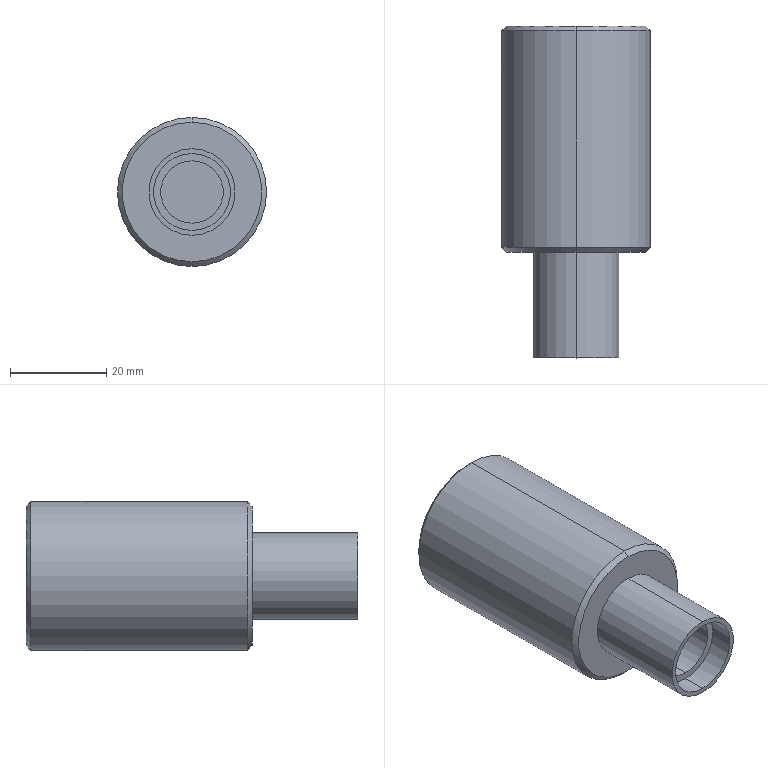Part | STEP file | PN_0009 Center JIG_Default | 1 solid | 17 faces | box 31 x 69 x 31 mm | volume 37981 mm3 | cylinder 8 | plane 5 | cone 4 | commonest cylinder face diameters 13 x2 16 x2 18 x2 31 x2
STEP:
#1=CARTESIAN_POINT('',(0.,0.,0.));
#2=DIRECTION('',(0.,0.,1.));
#3=DIRECTION('',(1.,0.,0.));
#4=AXIS2_PLACEMENT_3D('',#1,#2,#3);
#5=CARTESIAN_POINT('',(0.,22.,-14.5));
#6=VERTEX_POINT('',#5);
#7=CARTESIAN_POINT('',(0.,22.,14.5));
#8=VERTEX_POINT('',#7);
#9=CARTESIAN_POINT('',(0.,22.,0.));
#10=DIRECTION('',(0.,-1.,0.));
#11=DIRECTION('',(0.,0.,-1.));
#12=AXIS2_PLACEMENT_3D('',#9,#10,#11);
#13=CIRCLE('',#12,14.5);
#14=CARTESIAN_POINT('',(0.,22.,0.));
#15=DIRECTION('',(0.,1.,0.));
#16=DIRECTION('',(0.,0.,1.));
#17=AXIS2_PLACEMENT_3D('',#14,#15,#16);
#18=CONICAL_SURFACE('',#17,14.5,0.7854);
#19=CARTESIAN_POINT('',(3.142,0.));
#20=DIRECTION('',(-1.,0.));
#21=VECTOR('',#20,1.);
#22=LINE('',#19,#21);
#23=(GEOMETRIC_REPRESENTATION_CONTEXT(2)PARAMETRIC_REPRESENTATION_CONTEXT()REPRESENTATION_CONTEXT('',''));
#24=DEFINITIONAL_REPRESENTATION('',(#22),#23);
#25=PCURVE('',#18,#24);
#26=CARTESIAN_POINT('',(0.,22.,-15.5));
#27=DIRECTION('',(0.,-1.,0.));
#28=DIRECTION('',(0.,0.,-1.));
#29=AXIS2_PLACEMENT_3D('',#26,#27,#28);
#30=PLANE('',#29);
#31=CARTESIAN_POINT('',(-15.5,0.));
#32=DIRECTION('',(1.,0.));
#33=AXIS2_PLACEMENT_2D('',#31,#32);
#34=CIRCLE('',#33,14.5);
#35=(GEOMETRIC_REPRESENTATION_CONTEXT(2)PARAMETRIC_REPRESENTATION_CONTEXT()REPRESENTATION_CONTEXT('',''));
#36=DEFINITIONAL_REPRESENTATION('',(#34),#35);
#37=PCURVE('',#30,#36);
#38=SURFACE_CURVE('',#13,(#25,#37),.PCURVE_S1.);
#39=EDGE_CURVE('',#6,#8,#38,.T.);
#40=ORIENTED_EDGE('',*,*,#39,.F.);
#41=CARTESIAN_POINT('',(0.,23.,-15.5));
#42=VERTEX_POINT('',#41);
#43=CARTESIAN_POINT('',(0.,22.,-14.5));
#44=DIRECTION('',(0.,0.7071,-0.7071));
#45=VECTOR('',#44,1.);
#46=LINE('',#43,#45);
#47=CARTESIAN_POINT('',(3.142,0.));
#48=DIRECTION('',(0.,1.));
#49=VECTOR('',#48,1.);
#50=LINE('',#47,#49);
#51=(GEOMETRIC_REPRESENTATION_CONTEXT(2)PARAMETRIC_REPRESENTATION_CONTEXT()REPRESENTATION_CONTEXT('',''));
#52=DEFINITIONAL_REPRESENTATION('',(#50),#51);
#53=PCURVE('',#18,#52);
#54=CARTESIAN_POINT('',(0.,22.,0.));
#55=DIRECTION('',(0.,1.,0.));
#56=DIRECTION('',(0.,0.,1.));
#57=AXIS2_PLACEMENT_3D('',#54,#55,#56);
#58=CONICAL_SURFACE('',#57,14.5,0.7854);
#59=CARTESIAN_POINT('',(3.142,0.));
#60=DIRECTION('',(0.,1.));
#61=VECTOR('',#60,1.);
#62=LINE('',#59,#61);
#63=(GEOMETRIC_REPRESENTATION_CONTEXT(2)PARAMETRIC_REPRESENTATION_CONTEXT()REPRESENTATION_CONTEXT('',''));
#64=DEFINITIONAL_REPRESENTATION('',(#62),#63);
#65=PCURVE('',#58,#64);
#66=SURFACE_CURVE('',#46,(#53,#65),.PCURVE_S1.);
#67=EDGE_CURVE('',#6,#42,#66,.T.);
#68=ORIENTED_EDGE('',*,*,#67,.T.);
#69=CARTESIAN_POINT('',(0.,23.,15.5));
#70=VERTEX_POINT('',#69);
#71=CARTESIAN_POINT('',(0.,23.,0.));
#72=DIRECTION('',(0.,1.,0.));
#73=DIRECTION('',(0.,0.,-1.));
#74=AXIS2_PLACEMENT_3D('',#71,#72,#73);
#75=CIRCLE('',#74,15.5);
#76=CARTESIAN_POINT('',(-3.142,1.));
#77=DIRECTION('',(1.,0.));
#78=VECTOR('',#77,1.);
#79=LINE('',#76,#78);
#80=(GEOMETRIC_REPRESENTATION_CONTEXT(2)PARAMETRIC_REPRESENTATION_CONTEXT()REPRESENTATION_CONTEXT('',''));
#81=DEFINITIONAL_REPRESENTATION('',(#79),#80);
#82=PCURVE('',#18,#81);
#83=CARTESIAN_POINT('',(0.,-5.951,0.));
#84=DIRECTION('',(0.,-1.,0.));
#85=DIRECTION('',(0.,0.,-1.));
#86=AXIS2_PLACEMENT_3D('',#83,#84,#85);
#87=CYLINDRICAL_SURFACE('',#86,15.5);
#88=CARTESIAN_POINT('',(6.283,-28.951));
#89=DIRECTION('',(-1.,0.));
#90=VECTOR('',#89,1.);
#91=LINE('',#88,#90);
#92=(GEOMETRIC_REPRESENTATION_CONTEXT(2)PARAMETRIC_REPRESENTATION_CONTEXT()REPRESENTATION_CONTEXT('',''));
#93=DEFINITIONAL_REPRESENTATION('',(#91),#92);
#94=PCURVE('',#87,#93);
#95=SURFACE_CURVE('',#75,(#82,#94),.PCURVE_S1.);
#96=EDGE_CURVE('',#70,#42,#95,.T.);
#97=ORIENTED_EDGE('',*,*,#96,.F.);
#98=CARTESIAN_POINT('',(0.,22.,14.5));
#99=DIRECTION('',(0.,0.7071,0.7071));
#100=VECTOR('',#99,1.);
#101=LINE('',#98,#100);
#102=CARTESIAN_POINT('',(0.,0.));
#103=DIRECTION('',(0.,1.));
#104=VECTOR('',#103,1.);
#105=LINE('',#102,#104);
#106=(GEOMETRIC_REPRESENTATION_CONTEXT(2)PARAMETRIC_REPRESENTATION_CONTEXT()REPRESENTATION_CONTEXT('',''));
#107=DEFINITIONAL_REPRESENTATION('',(#105),#106);
#108=PCURVE('',#18,#107);
#109=CARTESIAN_POINT('',(6.283,0.));
#110=DIRECTION('',(0.,1.));
#111=VECTOR('',#110,1.);
#112=LINE('',#109,#111);
#113=(GEOMETRIC_REPRESENTATION_CONTEXT(2)PARAMETRIC_REPRESENTATION_CONTEXT()REPRESENTATION_CONTEXT('',''));
#114=DEFINITIONAL_REPRESENTATION('',(#112),#113);
#115=PCURVE('',#58,#114);
#116=SURFACE_CURVE('',#101,(#108,#115),.PCURVE_S1.);
#117=EDGE_CURVE('',#8,#70,#116,.T.);
#118=ORIENTED_EDGE('',*,*,#117,.F.);
#119=EDGE_LOOP('',(#40,#68,#97,#118));
#120=FACE_BOUND('',#119,.T.);
#121=ADVANCED_FACE('',(#120),#18,.T.);
#122=CARTESIAN_POINT('',(0.,69.,14.5));
#123=VERTEX_POINT('',#122);
#124=CARTESIAN_POINT('',(0.,69.,-14.5));
#125=VERTEX_POINT('',#124);
#126=CARTESIAN_POINT('',(0.,69.,0.));
#127=DIRECTION('',(0.,1.,0.));
#128=DIRECTION('',(0.,0.,1.));
#129=AXIS2_PLACEMENT_3D('',#126,#127,#128);
#130=CIRCLE('',#129,14.5);
#131=CARTESIAN_POINT('',(0.,68.,0.));
#132=DIRECTION('',(0.,-1.,0.));
#133=DIRECTION('',(0.,0.,-1.));
#134=AXIS2_PLACEMENT_3D('',#131,#132,#133);
#135=CONICAL_SURFACE('',#134,15.5,0.7854);
#136=CARTESIAN_POINT('',(3.142,-1.));
#137=DIRECTION('',(-1.,0.));
#138=VECTOR('',#137,1.);
#139=LINE('',#136,#138);
#140=(GEOMETRIC_REPRESENTATION_CONTEXT(2)PARAMETRIC_REPRESENTATION_CONTEXT()REPRESENTATION_CONTEXT('',''));
#141=DEFINITIONAL_REPRESENTATION('',(#139),#140);
#142=PCURVE('',#135,#141);
#143=CARTESIAN_POINT('',(0.,69.,-15.5));
#144=DIRECTION('',(0.,1.,0.));
#145=DIRECTION('',(0.,0.,1.));
#146=AXIS2_PLACEMENT_3D('',#143,#144,#145);
#147=PLANE('',#146);
#148=CARTESIAN_POINT('',(15.5,0.));
#149=DIRECTION('',(1.,0.));
#150=AXIS2_PLACEMENT_2D('',#148,#149);
#151=CIRCLE('',#150,14.5);
#152=(GEOMETRIC_REPRESENTATION_CONTEXT(2)PARAMETRIC_REPRESENTATION_CONTEXT()REPRESENTATION_CONTEXT('',''));
#153=DEFINITIONAL_REPRESENTATION('',(#151),#152);
#154=PCURVE('',#147,#153);
#155=SURFACE_CURVE('',#130,(#142,#154),.PCURVE_S1.);
#156=EDGE_CURVE('',#123,#125,#155,.T.);
#157=ORIENTED_EDGE('',*,*,#156,.F.);
#158=CARTESIAN_POINT('',(0.,68.,15.5));
#159=VERTEX_POINT('',#158);
#160=CARTESIAN_POINT('',(0.,68.,15.5));
#161=DIRECTION('',(0.,-0.7071,0.7071));
#162=VECTOR('',#161,1.);
#163=LINE('',#160,#162);
#164=CARTESIAN_POINT('',(3.142,0.));
#165=DIRECTION('',(0.,1.));
#166=VECTOR('',#165,1.);
#167=LINE('',#164,#166);
#168=(GEOMETRIC_REPRESENTATION_CONTEXT(2)PARAMETRIC_REPRESENTATION_CONTEXT()REPRESENTATION_CONTEXT('',''));
#169=DEFINITIONAL_REPRESENTATION('',(#167),#168);
#170=PCURVE('',#135,#169);
#171=CARTESIAN_POINT('',(0.,68.,0.));
#172=DIRECTION('',(0.,-1.,0.));
#173=DIRECTION('',(0.,0.,-1.));
#174=AXIS2_PLACEMENT_3D('',#171,#172,#173);
#175=CONICAL_SURFACE('',#174,15.5,0.7854);
#176=CARTESIAN_POINT('',(3.142,0.));
#177=DIRECTION('',(0.,1.));
#178=VECTOR('',#177,1.);
#179=LINE('',#176,#178);
#180=(GEOMETRIC_REPRESENTATION_CONTEXT(2)PARAMETRIC_REPRESENTATION_CONTEXT()REPRESENTATION_CONTEXT('',''));
#181=DEFINITIONAL_REPRESENTATION('',(#179),#180);
#182=PCURVE('',#175,#181);
#183=SURFACE_CURVE('',#163,(#170,#182),.PCURVE_S1.);
#184=EDGE_CURVE('',#123,#159,#183,.T.);
#185=ORIENTED_EDGE('',*,*,#184,.T.);
#186=CARTESIAN_POINT('',(0.,68.,-15.5));
#187=VERTEX_POINT('',#186);
#188=CARTESIAN_POINT('',(0.,68.,0.));
#189=DIRECTION('',(0.,-1.,0.));
#190=DIRECTION('',(0.,0.,1.));
#191=AXIS2_PLACEMENT_3D('',#188,#189,#190);
#192=CIRCLE('',#191,15.5);
#193=CARTESIAN_POINT('',(-3.142,0.));
#194=DIRECTION('',(1.,0.));
#195=VECTOR('',#194,1.);
#196=LINE('',#193,#195);
#197=(GEOMETRIC_REPRESENTATION_CONTEXT(2)PARAMETRIC_REPRESENTATION_CONTEXT()REPRESENTATION_CONTEXT('',''));
#198=DEFINITIONAL_REPRESENTATION('',(#196),#197);
#199=PCURVE('',#135,#198);
#200=CARTESIAN_POINT('',(-3.142,-73.951));
#201=DIRECTION('',(1.,0.));
#202=VECTOR('',#201,1.);
#203=LINE('',#200,#202);
#204=(GEOMETRIC_REPRESENTATION_CONTEXT(2)PARAMETRIC_REPRESENTATION_CONTEXT()REPRESENTATION_CONTEXT('',''));
#205=DEFINITIONAL_REPRESENTATION('',(#203),#204);
#206=PCURVE('',#87,#205);
#207=SURFACE_CURVE('',#192,(#199,#206),.PCURVE_S1.);
#208=EDGE_CURVE('',#187,#159,#207,.T.);
#209=ORIENTED_EDGE('',*,*,#208,.F.);
#210=CARTESIAN_POINT('',(0.,68.,-15.5));
#211=DIRECTION('',(0.,-0.7071,-0.7071));
#212=VECTOR('',#211,1.);
#213=LINE('',#210,#212);
#214=CARTESIAN_POINT('',(0.,0.));
#215=DIRECTION('',(0.,1.));
#216=VECTOR('',#215,1.);
#217=LINE('',#214,#216);
#218=(GEOMETRIC_REPRESENTATION_CONTEXT(2)PARAMETRIC_REPRESENTATION_CONTEXT()REPRESENTATION_CONTEXT('',''));
#219=DEFINITIONAL_REPRESENTATION('',(#217),#218);
#220=PCURVE('',#135,#219);
#221=CARTESIAN_POINT('',(6.283,0.));
#222=DIRECTION('',(0.,1.));
#223=VECTOR('',#222,1.);
#224=LINE('',#221,#223);
#225=(GEOMETRIC_REPRESENTATION_CONTEXT(2)PARAMETRIC_REPRESENTATION_CONTEXT()REPRESENTATION_CONTEXT('',''));
#226=DEFINITIONAL_REPRESENTATION('',(#224),#225);
#227=PCURVE('',#175,#226);
#228=SURFACE_CURVE('',#213,(#220,#227),.PCURVE_S1.);
#229=EDGE_CURVE('',#125,#187,#228,.T.);
#230=ORIENTED_EDGE('',*,*,#229,.F.);
#231=EDGE_LOOP('',(#157,#185,#209,#230));
#232=FACE_BOUND('',#231,.T.);
#233=ADVANCED_FACE('',(#232),#135,.T.);
#234=CARTESIAN_POINT('',(0.,20.,-6.5));
#235=VERTEX_POINT('',#234);
#236=CARTESIAN_POINT('',(0.,5.,-6.5));
#237=VERTEX_POINT('',#236);
#238=CARTESIAN_POINT('',(0.,20.,-6.5));
#239=DIRECTION('',(0.,-1.,0.));
#240=VECTOR('',#239,1.);
#241=LINE('',#238,#240);
#242=CARTESIAN_POINT('',(0.,20.,0.));
#243=DIRECTION('',(0.,-1.,0.));
#244=DIRECTION('',(0.,0.,-1.));
#245=AXIS2_PLACEMENT_3D('',#242,#243,#244);
#246=CYLINDRICAL_SURFACE('',#245,6.5);
#247=CARTESIAN_POINT('',(6.283,0.));
#248=DIRECTION('',(0.,1.));
#249=VECTOR('',#248,1.);
#250=LINE('',#247,#249);
#251=(GEOMETRIC_REPRESENTATION_CONTEXT(2)PARAMETRIC_REPRESENTATION_CONTEXT()REPRESENTATION_CONTEXT('',''));
#252=DEFINITIONAL_REPRESENTATION('',(#250),#251);
#253=PCURVE('',#246,#252);
#254=CARTESIAN_POINT('',(0.,20.,0.));
#255=DIRECTION('',(0.,-1.,0.));
#256=DIRECTION('',(0.,0.,-1.));
#257=AXIS2_PLACEMENT_3D('',#254,#255,#256);
#258=CYLINDRICAL_SURFACE('',#257,6.5);
#259=CARTESIAN_POINT('',(0.,0.));
#260=DIRECTION('',(0.,1.));
#261=VECTOR('',#260,1.);
#262=LINE('',#259,#261);
#263=(GEOMETRIC_REPRESENTATION_CONTEXT(2)PARAMETRIC_REPRESENTATION_CONTEXT()REPRESENTATION_CONTEXT('',''));
#264=DEFINITIONAL_REPRESENTATION('',(#262),#263);
#265=PCURVE('',#258,#264);
#266=SURFACE_CURVE('',#241,(#253,#265),.PCURVE_S1.);
#267=EDGE_CURVE('',#235,#237,#266,.T.);
#268=ORIENTED_EDGE('',*,*,#267,.T.);
#269=CARTESIAN_POINT('',(0.,5.,6.5));
#270=VERTEX_POINT('',#269);
#271=CARTESIAN_POINT('',(0.,5.,0.));
#272=DIRECTION('',(0.,-1.,0.));
#273=DIRECTION('',(0.,0.,-1.));
#274=AXIS2_PLACEMENT_3D('',#271,#272,#273);
#275=CIRCLE('',#274,6.5);
#276=CARTESIAN_POINT('',(0.,15.));
#277=DIRECTION('',(1.,0.));
#278=VECTOR('',#277,1.);
#279=LINE('',#276,#278);
#280=(GEOMETRIC_REPRESENTATION_CONTEXT(2)PARAMETRIC_REPRESENTATION_CONTEXT()REPRESENTATION_CONTEXT('',''));
#281=DEFINITIONAL_REPRESENTATION('',(#279),#280);
#282=PCURVE('',#246,#281);
#283=CARTESIAN_POINT('',(0.,5.,0.));
#284=DIRECTION('',(0.,-1.,0.));
#285=DIRECTION('',(0.,0.,-1.));
#286=AXIS2_PLACEMENT_3D('',#283,#284,#285);
#287=PLANE('',#286);
#288=CARTESIAN_POINT('',(0.,0.));
#289=DIRECTION('',(1.,0.));
#290=AXIS2_PLACEMENT_2D('',#288,#289);
#291=CIRCLE('',#290,6.5);
#292=(GEOMETRIC_REPRESENTATION_CONTEXT(2)PARAMETRIC_REPRESENTATION_CONTEXT()REPRESENTATION_CONTEXT('',''));
#293=DEFINITIONAL_REPRESENTATION('',(#291),#292);
#294=PCURVE('',#287,#293);
#295=SURFACE_CURVE('',#275,(#282,#294),.PCURVE_S1.);
#296=EDGE_CURVE('',#270,#237,#295,.T.);
#297=ORIENTED_EDGE('',*,*,#296,.F.);
#298=CARTESIAN_POINT('',(0.,20.,6.5));
#299=VERTEX_POINT('',#298);
#300=CARTESIAN_POINT('',(0.,20.,6.5));
#301=DIRECTION('',(0.,-1.,0.));
#302=VECTOR('',#301,1.);
#303=LINE('',#300,#302);
#304=CARTESIAN_POINT('',(3.142,0.));
#305=DIRECTION('',(0.,1.));
#306=VECTOR('',#305,1.);
#307=LINE('',#304,#306);
#308=(GEOMETRIC_REPRESENTATION_CONTEXT(2)PARAMETRIC_REPRESENTATION_CONTEXT()REPRESENTATION_CONTEXT('',''));
#309=DEFINITIONAL_REPRESENTATION('',(#307),#308);
#310=PCURVE('',#246,#309);
#311=CARTESIAN_POINT('',(3.142,0.));
#312=DIRECTION('',(0.,1.));
#313=VECTOR('',#312,1.);
#314=LINE('',#311,#313);
#315=(GEOMETRIC_REPRESENTATION_CONTEXT(2)PARAMETRIC_REPRESENTATION_CONTEXT()REPRESENTATION_CONTEXT('',''));
#316=DEFINITIONAL_REPRESENTATION('',(#314),#315);
#317=PCURVE('',#258,#316);
#318=SURFACE_CURVE('',#303,(#310,#317),.PCURVE_S1.);
#319=EDGE_CURVE('',#299,#270,#318,.T.);
#320=ORIENTED_EDGE('',*,*,#319,.F.);
#321=CARTESIAN_POINT('',(0.,20.,0.));
#322=DIRECTION('',(0.,-1.,0.));
#323=DIRECTION('',(0.,0.,-1.));
#324=AXIS2_PLACEMENT_3D('',#321,#322,#323);
#325=CIRCLE('',#324,6.5);
#326=CARTESIAN_POINT('',(0.,0.));
#327=DIRECTION('',(1.,0.));
#328=VECTOR('',#327,1.);
#329=LINE('',#326,#328);
#330=(GEOMETRIC_REPRESENTATION_CONTEXT(2)PARAMETRIC_REPRESENTATION_CONTEXT()REPRESENTATION_CONTEXT('',''));
#331=DEFINITIONAL_REPRESENTATION('',(#329),#330);
#332=PCURVE('',#246,#331);
#333=CARTESIAN_POINT('',(0.,20.,0.));
#334=DIRECTION('',(0.,-1.,0.));
#335=DIRECTION('',(0.,0.,-1.));
#336=AXIS2_PLACEMENT_3D('',#333,#334,#335);
#337=PLANE('',#336);
#338=CARTESIAN_POINT('',(0.,0.));
#339=DIRECTION('',(1.,0.));
#340=AXIS2_PLACEMENT_2D('',#338,#339);
#341=CIRCLE('',#340,6.5);
#342=(GEOMETRIC_REPRESENTATION_CONTEXT(2)PARAMETRIC_REPRESENTATION_CONTEXT()REPRESENTATION_CONTEXT('',''));
#343=DEFINITIONAL_REPRESENTATION('',(#341),#342);
#344=PCURVE('',#337,#343);
#345=SURFACE_CURVE('',#325,(#332,#344),.PCURVE_S1.);
#346=EDGE_CURVE('',#299,#235,#345,.T.);
#347=ORIENTED_EDGE('',*,*,#346,.T.);
#348=EDGE_LOOP('',(#268,#297,#320,#347));
#349=FACE_BOUND('',#348,.F.);
#350=ADVANCED_FACE('',(#349),#246,.F.);
#351=CARTESIAN_POINT('',(0.,5.,-8.));
#352=VERTEX_POINT('',#351);
#353=CARTESIAN_POINT('',(0.,0.,-8.));
#354=VERTEX_POINT('',#353);
#355=CARTESIAN_POINT('',(0.,5.,-8.));
#356=DIRECTION('',(0.,-1.,0.));
#357=VECTOR('',#356,1.);
#358=LINE('',#355,#357);
#359=CARTESIAN_POINT('',(0.,5.,0.));
#360=DIRECTION('',(0.,-1.,0.));
#361=DIRECTION('',(0.,0.,-1.));
#362=AXIS2_PLACEMENT_3D('',#359,#360,#361);
#363=CYLINDRICAL_SURFACE('',#362,8.);
#364=CARTESIAN_POINT('',(6.283,0.));
#365=DIRECTION('',(0.,1.));
#366=VECTOR('',#365,1.);
#367=LINE('',#364,#366);
#368=(GEOMETRIC_REPRESENTATION_CONTEXT(2)PARAMETRIC_REPRESENTATION_CONTEXT()REPRESENTATION_CONTEXT('',''));
#369=DEFINITIONAL_REPRESENTATION('',(#367),#368);
#370=PCURVE('',#363,#369);
#371=CARTESIAN_POINT('',(0.,5.,0.));
#372=DIRECTION('',(0.,-1.,0.));
#373=DIRECTION('',(0.,0.,-1.));
#374=AXIS2_PLACEMENT_3D('',#371,#372,#373);
#375=CYLINDRICAL_SURFACE('',#374,8.);
#376=CARTESIAN_POINT('',(0.,0.));
#377=DIRECTION('',(0.,1.));
#378=VECTOR('',#377,1.);
#379=LINE('',#376,#378);
#380=(GEOMETRIC_REPRESENTATION_CONTEXT(2)PARAMETRIC_REPRESENTATION_CONTEXT()REPRESENTATION_CONTEXT('',''));
#381=DEFINITIONAL_REPRESENTATION('',(#379),#380);
#382=PCURVE('',#375,#381);
#383=SURFACE_CURVE('',#358,(#370,#382),.PCURVE_S1.);
#384=EDGE_CURVE('',#352,#354,#383,.T.);
#385=ORIENTED_EDGE('',*,*,#384,.T.);
#386=CARTESIAN_POINT('',(0.,0.,8.));
#387=VERTEX_POINT('',#386);
#388=CARTESIAN_POINT('',(0.,0.,0.));
#389=DIRECTION('',(0.,-1.,0.));
#390=DIRECTION('',(0.,0.,-1.));
#391=AXIS2_PLACEMENT_3D('',#388,#389,#390);
#392=CIRCLE('',#391,8.);
#393=CARTESIAN_POINT('',(0.,5.));
#394=DIRECTION('',(1.,0.));
#395=VECTOR('',#394,1.);
#396=LINE('',#393,#395);
#397=(GEOMETRIC_REPRESENTATION_CONTEXT(2)PARAMETRIC_REPRESENTATION_CONTEXT()REPRESENTATION_CONTEXT('',''));
#398=DEFINITIONAL_REPRESENTATION('',(#396),#397);
#399=PCURVE('',#363,#398);
#400=CARTESIAN_POINT('',(0.,0.,-9.));
#401=DIRECTION('',(0.,-1.,0.));
#402=DIRECTION('',(0.,0.,-1.));
#403=AXIS2_PLACEMENT_3D('',#400,#401,#402);
#404=PLANE('',#403);
#405=CARTESIAN_POINT('',(-9.,0.));
#406=DIRECTION('',(1.,0.));
#407=AXIS2_PLACEMENT_2D('',#405,#406);
#408=CIRCLE('',#407,8.);
#409=(GEOMETRIC_REPRESENTATION_CONTEXT(2)PARAMETRIC_REPRESENTATION_CONTEXT()REPRESENTATION_CONTEXT('',''));
#410=DEFINITIONAL_REPRESENTATION('',(#408),#409);
#411=PCURVE('',#404,#410);
#412=SURFACE_CURVE('',#392,(#399,#411),.PCURVE_S1.);
#413=EDGE_CURVE('',#387,#354,#412,.T.);
#414=ORIENTED_EDGE('',*,*,#413,.F.);
#415=CARTESIAN_POINT('',(0.,5.,8.));
#416=VERTEX_POINT('',#415);
#417=CARTESIAN_POINT('',(0.,5.,8.));
#418=DIRECTION('',(0.,-1.,0.));
#419=VECTOR('',#418,1.);
#420=LINE('',#417,#419);
#421=CARTESIAN_POINT('',(3.142,0.));
#422=DIRECTION('',(0.,1.));
#423=VECTOR('',#422,1.);
#424=LINE('',#421,#423);
#425=(GEOMETRIC_REPRESENTATION_CONTEXT(2)PARAMETRIC_REPRESENTATION_CONTEXT()REPRESENTATION_CONTEXT('',''));
#426=DEFINITIONAL_REPRESENTATION('',(#424),#425);
#427=PCURVE('',#363,#426);
#428=CARTESIAN_POINT('',(3.142,0.));
#429=DIRECTION('',(0.,1.));
#430=VECTOR('',#429,1.);
#431=LINE('',#428,#430);
#432=(GEOMETRIC_REPRESENTATION_CONTEXT(2)PARAMETRIC_REPRESENTATION_CONTEXT()REPRESENTATION_CONTEXT('',''));
#433=DEFINITIONAL_REPRESENTATION('',(#431),#432);
#434=PCURVE('',#375,#433);
#435=SURFACE_CURVE('',#420,(#427,#434),.PCURVE_S1.);
#436=EDGE_CURVE('',#416,#387,#435,.T.);
#437=ORIENTED_EDGE('',*,*,#436,.F.);
#438=CARTESIAN_POINT('',(0.,5.,0.));
#439=DIRECTION('',(0.,-1.,0.));
#440=DIRECTION('',(0.,0.,-1.));
#441=AXIS2_PLACEMENT_3D('',#438,#439,#440);
#442=CIRCLE('',#441,8.);
#443=CARTESIAN_POINT('',(0.,0.));
#444=DIRECTION('',(1.,0.));
#445=VECTOR('',#444,1.);
#446=LINE('',#443,#445);
#447=(GEOMETRIC_REPRESENTATION_CONTEXT(2)PARAMETRIC_REPRESENTATION_CONTEXT()REPRESENTATION_CONTEXT('',''));
#448=DEFINITIONAL_REPRESENTATION('',(#446),#447);
#449=PCURVE('',#363,#448);
#450=CARTESIAN_POINT('',(0.,0.));
#451=DIRECTION('',(1.,0.));
#452=AXIS2_PLACEMENT_2D('',#450,#451);
#453=CIRCLE('',#452,8.);
#454=(GEOMETRIC_REPRESENTATION_CONTEXT(2)PARAMETRIC_REPRESENTATION_CONTEXT()REPRESENTATION_CONTEXT('',''));
#455=DEFINITIONAL_REPRESENTATION('',(#453),#454);
#456=PCURVE('',#287,#455);
#457=SURFACE_CURVE('',#442,(#449,#456),.PCURVE_S1.);
#458=EDGE_CURVE('',#416,#352,#457,.T.);
#459=ORIENTED_EDGE('',*,*,#458,.T.);
#460=EDGE_LOOP('',(#385,#414,#437,#459));
#461=FACE_BOUND('',#460,.F.);
#462=ADVANCED_FACE('',(#461),#363,.F.);
#463=ORIENTED_EDGE('',*,*,#208,.T.);
#464=CARTESIAN_POINT('',(0.,-5.951,15.5));
#465=DIRECTION('',(0.,-1.,0.));
#466=VECTOR('',#465,1.);
#467=LINE('',#464,#466);
#468=CARTESIAN_POINT('',(3.142,0.));
#469=DIRECTION('',(0.,1.));
#470=VECTOR('',#469,1.);
#471=LINE('',#468,#470);
#472=(GEOMETRIC_REPRESENTATION_CONTEXT(2)PARAMETRIC_REPRESENTATION_CONTEXT()REPRESENTATION_CONTEXT('',''));
#473=DEFINITIONAL_REPRESENTATION('',(#471),#472);
#474=PCURVE('',#87,#473);
#475=CARTESIAN_POINT('',(0.,-5.951,0.));
#476=DIRECTION('',(0.,-1.,0.));
#477=DIRECTION('',(0.,0.,-1.));
#478=AXIS2_PLACEMENT_3D('',#475,#476,#477);
#479=CYLINDRICAL_SURFACE('',#478,15.5);
#480=CARTESIAN_POINT('',(3.142,0.));
#481=DIRECTION('',(0.,1.));
#482=VECTOR('',#481,1.);
#483=LINE('',#480,#482);
#484=(GEOMETRIC_REPRESENTATION_CONTEXT(2)PARAMETRIC_REPRESENTATION_CONTEXT()REPRESENTATION_CONTEXT('',''));
#485=DEFINITIONAL_REPRESENTATION('',(#483),#484);
#486=PCURVE('',#479,#485);
#487=SURFACE_CURVE('',#467,(#474,#486),.PCURVE_S1.);
#488=EDGE_CURVE('',#159,#70,#487,.T.);
#489=ORIENTED_EDGE('',*,*,#488,.T.);
#490=ORIENTED_EDGE('',*,*,#96,.T.);
#491=CARTESIAN_POINT('',(0.,-5.951,-15.5));
#492=DIRECTION('',(0.,-1.,0.));
#493=VECTOR('',#492,1.);
#494=LINE('',#491,#493);
#495=CARTESIAN_POINT('',(0.,0.));
#496=DIRECTION('',(0.,1.));
#497=VECTOR('',#496,1.);
#498=LINE('',#495,#497);
#499=(GEOMETRIC_REPRESENTATION_CONTEXT(2)PARAMETRIC_REPRESENTATION_CONTEXT()REPRESENTATION_CONTEXT('',''));
#500=DEFINITIONAL_REPRESENTATION('',(#498),#499);
#501=PCURVE('',#87,#500);
#502=CARTESIAN_POINT('',(6.283,0.));
#503=DIRECTION('',(0.,1.));
#504=VECTOR('',#503,1.);
#505=LINE('',#502,#504);
#506=(GEOMETRIC_REPRESENTATION_CONTEXT(2)PARAMETRIC_REPRESENTATION_CONTEXT()REPRESENTATION_CONTEXT('',''));
#507=DEFINITIONAL_REPRESENTATION('',(#505),#506);
#508=PCURVE('',#479,#507);
#509=SURFACE_CURVE('',#494,(#501,#508),.PCURVE_S1.);
#510=EDGE_CURVE('',#187,#42,#509,.T.);
#511=ORIENTED_EDGE('',*,*,#510,.F.);
#512=EDGE_LOOP('',(#463,#489,#490,#511));
#513=FACE_BOUND('',#512,.T.);
#514=ADVANCED_FACE('',(#513),#87,.T.);
#515=CARTESIAN_POINT('',(0.,22.,-9.));
#516=VERTEX_POINT('',#515);
#517=CARTESIAN_POINT('',(0.,22.,9.));
#518=VERTEX_POINT('',#517);
#519=CARTESIAN_POINT('',(0.,22.,0.));
#520=DIRECTION('',(0.,-1.,0.));
#521=DIRECTION('',(0.,0.,-1.));
#522=AXIS2_PLACEMENT_3D('',#519,#520,#521);
#523=CIRCLE('',#522,9.);
#524=CARTESIAN_POINT('',(0.,-5.951,0.));
#525=DIRECTION('',(0.,-1.,0.));
#526=DIRECTION('',(0.,0.,-1.));
#527=AXIS2_PLACEMENT_3D('',#524,#525,#526);
#528=CYLINDRICAL_SURFACE('',#527,9.);
#529=CARTESIAN_POINT('',(0.,-27.951));
#530=DIRECTION('',(1.,0.));
#531=VECTOR('',#530,1.);
#532=LINE('',#529,#531);
#533=(GEOMETRIC_REPRESENTATION_CONTEXT(2)PARAMETRIC_REPRESENTATION_CONTEXT()REPRESENTATION_CONTEXT('',''));
#534=DEFINITIONAL_REPRESENTATION('',(#532),#533);
#535=PCURVE('',#528,#534);
#536=CARTESIAN_POINT('',(-15.5,0.));
#537=DIRECTION('',(1.,0.));
#538=AXIS2_PLACEMENT_2D('',#536,#537);
#539=CIRCLE('',#538,9.);
#540=(GEOMETRIC_REPRESENTATION_CONTEXT(2)PARAMETRIC_REPRESENTATION_CONTEXT()REPRESENTATION_CONTEXT('',''));
#541=DEFINITIONAL_REPRESENTATION('',(#539),#540);
#542=PCURVE('',#30,#541);
#543=SURFACE_CURVE('',#523,(#535,#542),.PCURVE_S1.);
#544=EDGE_CURVE('',#516,#518,#543,.T.);
#545=ORIENTED_EDGE('',*,*,#544,.T.);
#546=CARTESIAN_POINT('',(0.,0.,9.));
#547=VERTEX_POINT('',#546);
#548=CARTESIAN_POINT('',(0.,-5.951,9.));
#549=DIRECTION('',(0.,-1.,0.));
#550=VECTOR('',#549,1.);
#551=LINE('',#548,#550);
#552=CARTESIAN_POINT('',(3.142,0.));
#553=DIRECTION('',(0.,1.));
#554=VECTOR('',#553,1.);
#555=LINE('',#552,#554);
#556=(GEOMETRIC_REPRESENTATION_CONTEXT(2)PARAMETRIC_REPRESENTATION_CONTEXT()REPRESENTATION_CONTEXT('',''));
#557=DEFINITIONAL_REPRESENTATION('',(#555),#556);
#558=PCURVE('',#528,#557);
#559=CARTESIAN_POINT('',(0.,-5.951,0.));
#560=DIRECTION('',(0.,-1.,0.));
#561=DIRECTION('',(0.,0.,-1.));
#562=AXIS2_PLACEMENT_3D('',#559,#560,#561);
#563=CYLINDRICAL_SURFACE('',#562,9.);
#564=CARTESIAN_POINT('',(3.142,0.));
#565=DIRECTION('',(0.,1.));
#566=VECTOR('',#565,1.);
#567=LINE('',#564,#566);
#568=(GEOMETRIC_REPRESENTATION_CONTEXT(2)PARAMETRIC_REPRESENTATION_CONTEXT()REPRESENTATION_CONTEXT('',''));
#569=DEFINITIONAL_REPRESENTATION('',(#567),#568);
#570=PCURVE('',#563,#569);
#571=SURFACE_CURVE('',#551,(#558,#570),.PCURVE_S1.);
#572=EDGE_CURVE('',#518,#547,#571,.T.);
#573=ORIENTED_EDGE('',*,*,#572,.T.);
#574=CARTESIAN_POINT('',(0.,0.,-9.));
#575=VERTEX_POINT('',#574);
#576=CARTESIAN_POINT('',(0.,0.,0.));
#577=DIRECTION('',(0.,-1.,0.));
#578=DIRECTION('',(0.,0.,-1.));
#579=AXIS2_PLACEMENT_3D('',#576,#577,#578);
#580=CIRCLE('',#579,9.);
#581=CARTESIAN_POINT('',(0.,-5.951));
#582=DIRECTION('',(1.,0.));
#583=VECTOR('',#582,1.);
#584=LINE('',#581,#583);
#585=(GEOMETRIC_REPRESENTATION_CONTEXT(2)PARAMETRIC_REPRESENTATION_CONTEXT()REPRESENTATION_CONTEXT('',''));
#586=DEFINITIONAL_REPRESENTATION('',(#584),#585);
#587=PCURVE('',#528,#586);
#588=CARTESIAN_POINT('',(-9.,0.));
#589=DIRECTION('',(1.,0.));
#590=AXIS2_PLACEMENT_2D('',#588,#589);
#591=CIRCLE('',#590,9.);
#592=(GEOMETRIC_REPRESENTATION_CONTEXT(2)PARAMETRIC_REPRESENTATION_CONTEXT()REPRESENTATION_CONTEXT('',''));
#593=DEFINITIONAL_REPRESENTATION('',(#591),#592);
#594=PCURVE('',#404,#593);
#595=SURFACE_CURVE('',#580,(#587,#594),.PCURVE_S1.);
#596=EDGE_CURVE('',#575,#547,#595,.T.);
#597=ORIENTED_EDGE('',*,*,#596,.F.);
#598=CARTESIAN_POINT('',(0.,-5.951,-9.));
#599=DIRECTION('',(0.,-1.,0.));
#600=VECTOR('',#599,1.);
#601=LINE('',#598,#600);
#602=CARTESIAN_POINT('',(0.,0.));
#603=DIRECTION('',(0.,1.));
#604=VECTOR('',#603,1.);
#605=LINE('',#602,#604);
#606=(GEOMETRIC_REPRESENTATION_CONTEXT(2)PARAMETRIC_REPRESENTATION_CONTEXT()REPRESENTATION_CONTEXT('',''));
#607=DEFINITIONAL_REPRESENTATION('',(#605),#606);
#608=PCURVE('',#528,#607);
#609=CARTESIAN_POINT('',(6.283,0.));
#610=DIRECTION('',(0.,1.));
#611=VECTOR('',#610,1.);
#612=LINE('',#609,#611);
#613=(GEOMETRIC_REPRESENTATION_CONTEXT(2)PARAMETRIC_REPRESENTATION_CONTEXT()REPRESENTATION_CONTEXT('',''));
#614=DEFINITIONAL_REPRESENTATION('',(#612),#613);
#615=PCURVE('',#563,#614);
#616=SURFACE_CURVE('',#601,(#608,#615),.PCURVE_S1.);
#617=EDGE_CURVE('',#516,#575,#616,.T.);
#618=ORIENTED_EDGE('',*,*,#617,.F.);
#619=EDGE_LOOP('',(#545,#573,#597,#618));
#620=FACE_BOUND('',#619,.T.);
#621=ADVANCED_FACE('',(#620),#528,.T.);
#622=CARTESIAN_POINT('',(0.,0.,0.));
#623=DIRECTION('',(0.,-1.,0.));
#624=DIRECTION('',(0.,0.,-1.));
#625=AXIS2_PLACEMENT_3D('',#622,#623,#624);
#626=CIRCLE('',#625,8.);
#627=CARTESIAN_POINT('',(-9.,0.));
#628=DIRECTION('',(1.,0.));
#629=AXIS2_PLACEMENT_2D('',#627,#628);
#630=CIRCLE('',#629,8.);
#631=(GEOMETRIC_REPRESENTATION_CONTEXT(2)PARAMETRIC_REPRESENTATION_CONTEXT()REPRESENTATION_CONTEXT('',''));
#632=DEFINITIONAL_REPRESENTATION('',(#630),#631);
#633=PCURVE('',#404,#632);
#634=CARTESIAN_POINT('',(0.,5.));
#635=DIRECTION('',(1.,0.));
#636=VECTOR('',#635,1.);
#637=LINE('',#634,#636);
#638=(GEOMETRIC_REPRESENTATION_CONTEXT(2)PARAMETRIC_REPRESENTATION_CONTEXT()REPRESENTATION_CONTEXT('',''));
#639=DEFINITIONAL_REPRESENTATION('',(#637),#638);
#640=PCURVE('',#375,#639);
#641=SURFACE_CURVE('',#626,(#633,#640),.PCURVE_S1.);
#642=EDGE_CURVE('',#354,#387,#641,.T.);
#643=ORIENTED_EDGE('',*,*,#642,.F.);
#644=ORIENTED_EDGE('',*,*,#413,.F.);
#645=EDGE_LOOP('',(#643,#644));
#646=FACE_BOUND('',#645,.T.);
#647=ORIENTED_EDGE('',*,*,#596,.T.);
#648=CARTESIAN_POINT('',(0.,0.,0.));
#649=DIRECTION('',(0.,-1.,0.));
#650=DIRECTION('',(0.,0.,-1.));
#651=AXIS2_PLACEMENT_3D('',#648,#649,#650);
#652=CIRCLE('',#651,9.);
#653=CARTESIAN_POINT('',(-9.,0.));
#654=DIRECTION('',(1.,0.));
#655=AXIS2_PLACEMENT_2D('',#653,#654);
#656=CIRCLE('',#655,9.);
#657=(GEOMETRIC_REPRESENTATION_CONTEXT(2)PARAMETRIC_REPRESENTATION_CONTEXT()REPRESENTATION_CONTEXT('',''));
#658=DEFINITIONAL_REPRESENTATION('',(#656),#657);
#659=PCURVE('',#404,#658);
#660=CARTESIAN_POINT('',(0.,-5.951));
#661=DIRECTION('',(1.,0.));
#662=VECTOR('',#661,1.);
#663=LINE('',#660,#662);
#664=(GEOMETRIC_REPRESENTATION_CONTEXT(2)PARAMETRIC_REPRESENTATION_CONTEXT()REPRESENTATION_CONTEXT('',''));
#665=DEFINITIONAL_REPRESENTATION('',(#663),#664);
#666=PCURVE('',#563,#665);
#667=SURFACE_CURVE('',#652,(#659,#666),.PCURVE_S1.);
#668=EDGE_CURVE('',#547,#575,#667,.T.);
#669=ORIENTED_EDGE('',*,*,#668,.T.);
#670=EDGE_LOOP('',(#647,#669));
#671=FACE_BOUND('',#670,.T.);
#672=ADVANCED_FACE('',(#646,#671),#404,.T.);
#673=ORIENTED_EDGE('',*,*,#572,.F.);
#674=CARTESIAN_POINT('',(0.,22.,0.));
#675=DIRECTION('',(0.,-1.,0.));
#676=DIRECTION('',(0.,0.,-1.));
#677=AXIS2_PLACEMENT_3D('',#674,#675,#676);
#678=CIRCLE('',#677,9.);
#679=CARTESIAN_POINT('',(0.,-27.951));
#680=DIRECTION('',(1.,0.));
#681=VECTOR('',#680,1.);
#682=LINE('',#679,#681);
#683=(GEOMETRIC_REPRESENTATION_CONTEXT(2)PARAMETRIC_REPRESENTATION_CONTEXT()REPRESENTATION_CONTEXT('',''));
#684=DEFINITIONAL_REPRESENTATION('',(#682),#683);
#685=PCURVE('',#563,#684);
#686=CARTESIAN_POINT('',(-15.5,0.));
#687=DIRECTION('',(1.,0.));
#688=AXIS2_PLACEMENT_2D('',#686,#687);
#689=CIRCLE('',#688,9.);
#690=(GEOMETRIC_REPRESENTATION_CONTEXT(2)PARAMETRIC_REPRESENTATION_CONTEXT()REPRESENTATION_CONTEXT('',''));
#691=DEFINITIONAL_REPRESENTATION('',(#689),#690);
#692=PCURVE('',#30,#691);
#693=SURFACE_CURVE('',#678,(#685,#692),.PCURVE_S1.);
#694=EDGE_CURVE('',#518,#516,#693,.T.);
#695=ORIENTED_EDGE('',*,*,#694,.T.);
#696=ORIENTED_EDGE('',*,*,#617,.T.);
#697=ORIENTED_EDGE('',*,*,#668,.F.);
#698=EDGE_LOOP('',(#673,#695,#696,#697));
#699=FACE_BOUND('',#698,.T.);
#700=ADVANCED_FACE('',(#699),#563,.T.);
#701=CARTESIAN_POINT('',(0.,22.,0.));
#702=DIRECTION('',(0.,-1.,0.));
#703=DIRECTION('',(0.,0.,-1.));
#704=AXIS2_PLACEMENT_3D('',#701,#702,#703);
#705=CIRCLE('',#704,14.5);
#706=CARTESIAN_POINT('',(-15.5,0.));
#707=DIRECTION('',(1.,0.));
#708=AXIS2_PLACEMENT_2D('',#706,#707);
#709=CIRCLE('',#708,14.5);
#710=(GEOMETRIC_REPRESENTATION_CONTEXT(2)PARAMETRIC_REPRESENTATION_CONTEXT()REPRESENTATION_CONTEXT('',''));
#711=DEFINITIONAL_REPRESENTATION('',(#709),#710);
#712=PCURVE('',#30,#711);
#713=CARTESIAN_POINT('',(9.425,0.));
#714=DIRECTION('',(-1.,0.));
#715=VECTOR('',#714,1.);
#716=LINE('',#713,#715);
#717=(GEOMETRIC_REPRESENTATION_CONTEXT(2)PARAMETRIC_REPRESENTATION_CONTEXT()REPRESENTATION_CONTEXT('',''));
#718=DEFINITIONAL_REPRESENTATION('',(#716),#717);
#719=PCURVE('',#58,#718);
#720=SURFACE_CURVE('',#705,(#712,#719),.PCURVE_S1.);
#721=EDGE_CURVE('',#8,#6,#720,.T.);
#722=ORIENTED_EDGE('',*,*,#721,.T.);
#723=ORIENTED_EDGE('',*,*,#39,.T.);
#724=EDGE_LOOP('',(#722,#723));
#725=FACE_BOUND('',#724,.T.);
#726=ORIENTED_EDGE('',*,*,#544,.F.);
#727=ORIENTED_EDGE('',*,*,#694,.F.);
#728=EDGE_LOOP('',(#726,#727));
#729=FACE_BOUND('',#728,.T.);
#730=ADVANCED_FACE('',(#725,#729),#30,.T.);
#731=ORIENTED_EDGE('',*,*,#488,.F.);
#732=CARTESIAN_POINT('',(0.,68.,0.));
#733=DIRECTION('',(0.,-1.,0.));
#734=DIRECTION('',(0.,0.,1.));
#735=AXIS2_PLACEMENT_3D('',#732,#733,#734);
#736=CIRCLE('',#735,15.5);
#737=CARTESIAN_POINT('',(3.142,-73.951));
#738=DIRECTION('',(1.,0.));
#739=VECTOR('',#738,1.);
#740=LINE('',#737,#739);
#741=(GEOMETRIC_REPRESENTATION_CONTEXT(2)PARAMETRIC_REPRESENTATION_CONTEXT()REPRESENTATION_CONTEXT('',''));
#742=DEFINITIONAL_REPRESENTATION('',(#740),#741);
#743=PCURVE('',#479,#742);
#744=CARTESIAN_POINT('',(3.142,0.));
#745=DIRECTION('',(1.,0.));
#746=VECTOR('',#745,1.);
#747=LINE('',#744,#746);
#748=(GEOMETRIC_REPRESENTATION_CONTEXT(2)PARAMETRIC_REPRESENTATION_CONTEXT()REPRESENTATION_CONTEXT('',''));
#749=DEFINITIONAL_REPRESENTATION('',(#747),#748);
#750=PCURVE('',#175,#749);
#751=SURFACE_CURVE('',#736,(#743,#750),.PCURVE_S1.);
#752=EDGE_CURVE('',#159,#187,#751,.T.);
#753=ORIENTED_EDGE('',*,*,#752,.T.);
#754=ORIENTED_EDGE('',*,*,#510,.T.);
#755=CARTESIAN_POINT('',(0.,23.,0.));
#756=DIRECTION('',(0.,1.,0.));
#757=DIRECTION('',(0.,0.,-1.));
#758=AXIS2_PLACEMENT_3D('',#755,#756,#757);
#759=CIRCLE('',#758,15.5);
#760=CARTESIAN_POINT('',(6.283,-28.951));
#761=DIRECTION('',(-1.,0.));
#762=VECTOR('',#761,1.);
#763=LINE('',#760,#762);
#764=(GEOMETRIC_REPRESENTATION_CONTEXT(2)PARAMETRIC_REPRESENTATION_CONTEXT()REPRESENTATION_CONTEXT('',''));
#765=DEFINITIONAL_REPRESENTATION('',(#763),#764);
#766=PCURVE('',#479,#765);
#767=CARTESIAN_POINT('',(3.142,1.));
#768=DIRECTION('',(1.,0.));
#769=VECTOR('',#768,1.);
#770=LINE('',#767,#769);
#771=(GEOMETRIC_REPRESENTATION_CONTEXT(2)PARAMETRIC_REPRESENTATION_CONTEXT()REPRESENTATION_CONTEXT('',''));
#772=DEFINITIONAL_REPRESENTATION('',(#770),#771);
#773=PCURVE('',#58,#772);
#774=SURFACE_CURVE('',#759,(#766,#773),.PCURVE_S1.);
#775=EDGE_CURVE('',#42,#70,#774,.T.);
#776=ORIENTED_EDGE('',*,*,#775,.T.);
#777=EDGE_LOOP('',(#731,#753,#754,#776));
#778=FACE_BOUND('',#777,.T.);
#779=ADVANCED_FACE('',(#778),#479,.T.);
#780=CARTESIAN_POINT('',(0.,69.,0.));
#781=DIRECTION('',(0.,1.,0.));
#782=DIRECTION('',(0.,0.,1.));
#783=AXIS2_PLACEMENT_3D('',#780,#781,#782);
#784=CIRCLE('',#783,14.5);
#785=CARTESIAN_POINT('',(15.5,0.));
#786=DIRECTION('',(1.,0.));
#787=AXIS2_PLACEMENT_2D('',#785,#786);
#788=CIRCLE('',#787,14.5);
#789=(GEOMETRIC_REPRESENTATION_CONTEXT(2)PARAMETRIC_REPRESENTATION_CONTEXT()REPRESENTATION_CONTEXT('',''));
#790=DEFINITIONAL_REPRESENTATION('',(#788),#789);
#791=PCURVE('',#147,#790);
#792=CARTESIAN_POINT('',(9.425,-1.));
#793=DIRECTION('',(-1.,0.));
#794=VECTOR('',#793,1.);
#795=LINE('',#792,#794);
#796=(GEOMETRIC_REPRESENTATION_CONTEXT(2)PARAMETRIC_REPRESENTATION_CONTEXT()REPRESENTATION_CONTEXT('',''));
#797=DEFINITIONAL_REPRESENTATION('',(#795),#796);
#798=PCURVE('',#175,#797);
#799=SURFACE_CURVE('',#784,(#791,#798),.PCURVE_S1.);
#800=EDGE_CURVE('',#125,#123,#799,.T.);
#801=ORIENTED_EDGE('',*,*,#800,.T.);
#802=ORIENTED_EDGE('',*,*,#156,.T.);
#803=EDGE_LOOP('',(#801,#802));
#804=FACE_BOUND('',#803,.T.);
#805=ADVANCED_FACE('',(#804),#147,.T.);
#806=ORIENTED_EDGE('',*,*,#642,.F.);
#807=ORIENTED_EDGE('',*,*,#384,.F.);
#808=CARTESIAN_POINT('',(0.,5.,0.));
#809=DIRECTION('',(0.,-1.,0.));
#810=DIRECTION('',(0.,0.,-1.));
#811=AXIS2_PLACEMENT_3D('',#808,#809,#810);
#812=CIRCLE('',#811,8.);
#813=CARTESIAN_POINT('',(0.,0.));
#814=DIRECTION('',(1.,0.));
#815=VECTOR('',#814,1.);
#816=LINE('',#813,#815);
#817=(GEOMETRIC_REPRESENTATION_CONTEXT(2)PARAMETRIC_REPRESENTATION_CONTEXT()REPRESENTATION_CONTEXT('',''));
#818=DEFINITIONAL_REPRESENTATION('',(#816),#817);
#819=PCURVE('',#375,#818);
#820=CARTESIAN_POINT('',(0.,0.));
#821=DIRECTION('',(1.,0.));
#822=AXIS2_PLACEMENT_2D('',#820,#821);
#823=CIRCLE('',#822,8.);
#824=(GEOMETRIC_REPRESENTATION_CONTEXT(2)PARAMETRIC_REPRESENTATION_CONTEXT()REPRESENTATION_CONTEXT('',''));
#825=DEFINITIONAL_REPRESENTATION('',(#823),#824);
#826=PCURVE('',#287,#825);
#827=SURFACE_CURVE('',#812,(#819,#826),.PCURVE_S1.);
#828=EDGE_CURVE('',#352,#416,#827,.T.);
#829=ORIENTED_EDGE('',*,*,#828,.T.);
#830=ORIENTED_EDGE('',*,*,#436,.T.);
#831=EDGE_LOOP('',(#806,#807,#829,#830));
#832=FACE_BOUND('',#831,.F.);
#833=ADVANCED_FACE('',(#832),#375,.F.);
#834=CARTESIAN_POINT('',(0.,5.,0.));
#835=DIRECTION('',(0.,-1.,0.));
#836=DIRECTION('',(0.,0.,-1.));
#837=AXIS2_PLACEMENT_3D('',#834,#835,#836);
#838=CIRCLE('',#837,6.5);
#839=CARTESIAN_POINT('',(0.,0.));
#840=DIRECTION('',(1.,0.));
#841=AXIS2_PLACEMENT_2D('',#839,#840);
#842=CIRCLE('',#841,6.5);
#843=(GEOMETRIC_REPRESENTATION_CONTEXT(2)PARAMETRIC_REPRESENTATION_CONTEXT()REPRESENTATION_CONTEXT('',''));
#844=DEFINITIONAL_REPRESENTATION('',(#842),#843);
#845=PCURVE('',#287,#844);
#846=CARTESIAN_POINT('',(0.,15.));
#847=DIRECTION('',(1.,0.));
#848=VECTOR('',#847,1.);
#849=LINE('',#846,#848);
#850=(GEOMETRIC_REPRESENTATION_CONTEXT(2)PARAMETRIC_REPRESENTATION_CONTEXT()REPRESENTATION_CONTEXT('',''));
#851=DEFINITIONAL_REPRESENTATION('',(#849),#850);
#852=PCURVE('',#258,#851);
#853=SURFACE_CURVE('',#838,(#845,#852),.PCURVE_S1.);
#854=EDGE_CURVE('',#237,#270,#853,.T.);
#855=ORIENTED_EDGE('',*,*,#854,.F.);
#856=ORIENTED_EDGE('',*,*,#296,.F.);
#857=EDGE_LOOP('',(#855,#856));
#858=FACE_BOUND('',#857,.T.);
#859=ORIENTED_EDGE('',*,*,#828,.T.);
#860=ORIENTED_EDGE('',*,*,#458,.T.);
#861=EDGE_LOOP('',(#859,#860));
#862=FACE_BOUND('',#861,.T.);
#863=ADVANCED_FACE('',(#858,#862),#287,.T.);
#864=ORIENTED_EDGE('',*,*,#854,.F.);
#865=ORIENTED_EDGE('',*,*,#267,.F.);
#866=CARTESIAN_POINT('',(0.,20.,0.));
#867=DIRECTION('',(0.,-1.,0.));
#868=DIRECTION('',(0.,0.,-1.));
#869=AXIS2_PLACEMENT_3D('',#866,#867,#868);
#870=CIRCLE('',#869,6.5);
#871=CARTESIAN_POINT('',(0.,0.));
#872=DIRECTION('',(1.,0.));
#873=VECTOR('',#872,1.);
#874=LINE('',#871,#873);
#875=(GEOMETRIC_REPRESENTATION_CONTEXT(2)PARAMETRIC_REPRESENTATION_CONTEXT()REPRESENTATION_CONTEXT('',''));
#876=DEFINITIONAL_REPRESENTATION('',(#874),#875);
#877=PCURVE('',#258,#876);
#878=CARTESIAN_POINT('',(0.,0.));
#879=DIRECTION('',(1.,0.));
#880=AXIS2_PLACEMENT_2D('',#878,#879);
#881=CIRCLE('',#880,6.5);
#882=(GEOMETRIC_REPRESENTATION_CONTEXT(2)PARAMETRIC_REPRESENTATION_CONTEXT()REPRESENTATION_CONTEXT('',''));
#883=DEFINITIONAL_REPRESENTATION('',(#881),#882);
#884=PCURVE('',#337,#883);
#885=SURFACE_CURVE('',#870,(#877,#884),.PCURVE_S1.);
#886=EDGE_CURVE('',#235,#299,#885,.T.);
#887=ORIENTED_EDGE('',*,*,#886,.T.);
#888=ORIENTED_EDGE('',*,*,#319,.T.);
#889=EDGE_LOOP('',(#864,#865,#887,#888));
#890=FACE_BOUND('',#889,.F.);
#891=ADVANCED_FACE('',(#890),#258,.F.);
#892=ORIENTED_EDGE('',*,*,#886,.T.);
#893=ORIENTED_EDGE('',*,*,#346,.T.);
#894=EDGE_LOOP('',(#892,#893));
#895=FACE_BOUND('',#894,.T.);
#896=ADVANCED_FACE('',(#895),#337,.T.);
#897=ORIENTED_EDGE('',*,*,#184,.F.);
#898=ORIENTED_EDGE('',*,*,#800,.F.);
#899=ORIENTED_EDGE('',*,*,#229,.T.);
#900=ORIENTED_EDGE('',*,*,#752,.F.);
#901=EDGE_LOOP('',(#897,#898,#899,#900));
#902=FACE_BOUND('',#901,.T.);
#903=ADVANCED_FACE('',(#902),#175,.T.);
#904=ORIENTED_EDGE('',*,*,#67,.F.);
#905=ORIENTED_EDGE('',*,*,#721,.F.);
#906=ORIENTED_EDGE('',*,*,#117,.T.);
#907=ORIENTED_EDGE('',*,*,#775,.F.);
#908=EDGE_LOOP('',(#904,#905,#906,#907));
#909=FACE_BOUND('',#908,.T.);
#910=ADVANCED_FACE('',(#909),#58,.T.);
#911=CLOSED_SHELL('',(#121,#233,#350,#462,#514,#621,#672,#700,#730,#779,#805,#833,#863,#891,#896,#903,#910));
#912=MANIFOLD_SOLID_BREP('',#911);
#913=(LENGTH_UNIT()NAMED_UNIT(*)SI_UNIT(.MILLI.,.METRE.));
#914=UNCERTAINTY_MEASURE_WITH_UNIT(LENGTH_MEASURE(0.0000001),#913,'','');
#915=(NAMED_UNIT(*)PLANE_ANGLE_UNIT()SI_UNIT($,.RADIAN.));
#916=(NAMED_UNIT(*)SI_UNIT($,.STERADIAN.)SOLID_ANGLE_UNIT());
#917=(GEOMETRIC_REPRESENTATION_CONTEXT(3)GLOBAL_UNCERTAINTY_ASSIGNED_CONTEXT((#914))GLOBAL_UNIT_ASSIGNED_CONTEXT((#913,#915,#916))REPRESENTATION_CONTEXT('',''));
#918=ADVANCED_BREP_SHAPE_REPRESENTATION('',(#4,#912),#917);